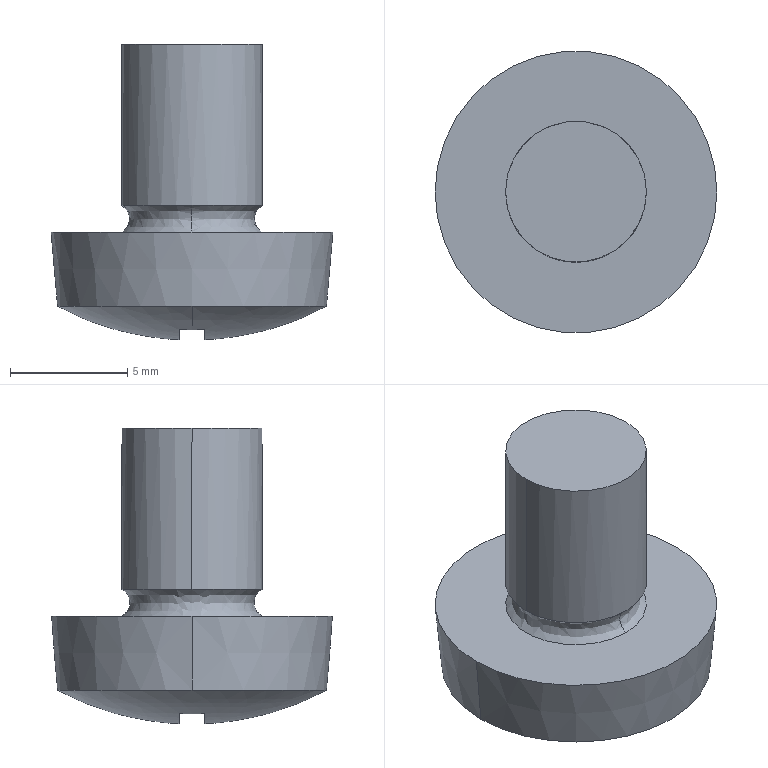Part | SolidWorks | features BaseBody 1 | 1 solid | 23 faces | box 12 x 12 x 12.575 mm | volume 614.773 mm3 | plane 15 | spline 4 | cone 2 | cylinder 2 | commonest cylinder face diameters 6 x2
STEP:
#1=CARTESIAN_POINT('',(480.537,34.715,-66.134));
#2=VERTEX_POINT('',#1);
#3=CARTESIAN_POINT('',(480.537,40.715,-66.134));
#4=VERTEX_POINT('',#3);
#5=CARTESIAN_POINT('',(480.537,37.715,-66.134));
#6=DIRECTION('',(-0.000000013,0.,1.));
#7=DIRECTION('',(-1.,0.,-0.000000013));
#8=AXIS2_PLACEMENT_3D('',#5,#6,#7);
#9=CIRCLE('',#8,3.);
#10=EDGE_CURVE('',#2,#4,#9,.T.);
#11=ORIENTED_EDGE('',*,*,#10,.T.);
#12=CARTESIAN_POINT('',(480.537,40.715,-64.991));
#13=VERTEX_POINT('',#12);
#14=CARTESIAN_POINT('',(480.537,40.715,-66.134));
#15=CARTESIAN_POINT('',(480.537,40.668,-66.111));
#16=CARTESIAN_POINT('',(480.537,40.572,-66.049));
#17=CARTESIAN_POINT('',(480.537,40.454,-65.917));
#18=CARTESIAN_POINT('',(480.537,40.375,-65.747));
#19=CARTESIAN_POINT('',(480.537,40.348,-65.563));
#20=CARTESIAN_POINT('',(480.537,40.375,-65.378));
#21=CARTESIAN_POINT('',(480.537,40.454,-65.208));
#22=CARTESIAN_POINT('',(480.537,40.572,-65.076));
#23=CARTESIAN_POINT('',(480.537,40.668,-65.014));
#24=CARTESIAN_POINT('',(480.537,40.715,-64.991));
#25=B_SPLINE_CURVE_WITH_KNOTS('',3,(#14,#15,#16,#17,#18,#19,#20,#21,#22,#23,#24),.UNSPECIFIED.,.F.,.F.,(4,1,1,1,1,1,1,1,4),(0.01923,0.125,0.25,0.375,0.5,0.625,0.75,0.875,0.9808),.UNSPECIFIED.);
#26=EDGE_CURVE('',#4,#13,#25,.T.);
#27=ORIENTED_EDGE('',*,*,#26,.T.);
#28=CARTESIAN_POINT('',(483.537,37.715,-64.991));
#29=VERTEX_POINT('',#28);
#30=CARTESIAN_POINT('',(480.537,37.715,-64.991));
#31=DIRECTION('',(0.000000013,0.,-1.));
#32=DIRECTION('',(0.,-1.,0.));
#33=AXIS2_PLACEMENT_3D('',#30,#31,#32);
#34=CIRCLE('',#33,3.);
#35=EDGE_CURVE('',#13,#29,#34,.T.);
#36=ORIENTED_EDGE('',*,*,#35,.T.);
#37=CARTESIAN_POINT('',(480.537,34.715,-64.991));
#38=VERTEX_POINT('',#37);
#39=CARTESIAN_POINT('',(480.537,37.715,-64.991));
#40=DIRECTION('',(0.000000013,0.,-1.));
#41=DIRECTION('',(0.,-1.,0.));
#42=AXIS2_PLACEMENT_3D('',#39,#40,#41);
#43=CIRCLE('',#42,3.);
#44=EDGE_CURVE('',#29,#38,#43,.T.);
#45=ORIENTED_EDGE('',*,*,#44,.T.);
#46=CARTESIAN_POINT('',(480.537,34.715,-66.134));
#47=CARTESIAN_POINT('',(480.537,34.762,-66.111));
#48=CARTESIAN_POINT('',(480.537,34.858,-66.049));
#49=CARTESIAN_POINT('',(480.537,34.976,-65.917));
#50=CARTESIAN_POINT('',(480.537,35.055,-65.747));
#51=CARTESIAN_POINT('',(480.537,35.082,-65.563));
#52=CARTESIAN_POINT('',(480.537,35.055,-65.378));
#53=CARTESIAN_POINT('',(480.537,34.976,-65.208));
#54=CARTESIAN_POINT('',(480.537,34.858,-65.076));
#55=CARTESIAN_POINT('',(480.537,34.762,-65.014));
#56=CARTESIAN_POINT('',(480.537,34.715,-64.991));
#57=B_SPLINE_CURVE_WITH_KNOTS('',3,(#46,#47,#48,#49,#50,#51,#52,#53,#54,#55,#56),.UNSPECIFIED.,.F.,.F.,(4,1,1,1,1,1,1,1,4),(0.01923,0.125,0.25,0.375,0.5,0.625,0.75,0.875,0.9808),.UNSPECIFIED.);
#58=EDGE_CURVE('',#2,#38,#57,.T.);
#59=ORIENTED_EDGE('',*,*,#58,.F.);
#60=EDGE_LOOP('',(#11,#27,#36,#45,#59));
#61=FACE_OUTER_BOUND('',#60,.T.);
#62=CARTESIAN_POINT('',(480.537,40.715,-66.134));
#63=CARTESIAN_POINT('',(482.294,40.715,-66.134));
#64=CARTESIAN_POINT('',(483.537,39.472,-66.134));
#65=CARTESIAN_POINT('',(483.537,37.715,-66.134));
#66=CARTESIAN_POINT('',(483.537,35.957,-66.134));
#67=CARTESIAN_POINT('',(482.294,34.715,-66.134));
#68=CARTESIAN_POINT('',(480.537,34.715,-66.134));
#69=CARTESIAN_POINT('',(480.537,40.668,-66.111));
#70=CARTESIAN_POINT('',(482.267,40.668,-66.111));
#71=CARTESIAN_POINT('',(483.49,39.445,-66.111));
#72=CARTESIAN_POINT('',(483.49,37.715,-66.111));
#73=CARTESIAN_POINT('',(483.49,35.985,-66.111));
#74=CARTESIAN_POINT('',(482.267,34.762,-66.111));
#75=CARTESIAN_POINT('',(480.537,34.762,-66.111));
#76=CARTESIAN_POINT('',(480.537,40.572,-66.049));
#77=CARTESIAN_POINT('',(482.21,40.572,-66.049));
#78=CARTESIAN_POINT('',(483.394,39.388,-66.049));
#79=CARTESIAN_POINT('',(483.394,37.715,-66.049));
#80=CARTESIAN_POINT('',(483.394,36.041,-66.049));
#81=CARTESIAN_POINT('',(482.21,34.858,-66.049));
#82=CARTESIAN_POINT('',(480.537,34.858,-66.049));
#83=CARTESIAN_POINT('',(480.537,40.454,-65.917));
#84=CARTESIAN_POINT('',(482.141,40.454,-65.917));
#85=CARTESIAN_POINT('',(483.276,39.319,-65.917));
#86=CARTESIAN_POINT('',(483.276,37.715,-65.917));
#87=CARTESIAN_POINT('',(483.276,36.11,-65.917));
#88=CARTESIAN_POINT('',(482.141,34.976,-65.917));
#89=CARTESIAN_POINT('',(480.537,34.976,-65.917));
#90=CARTESIAN_POINT('',(480.537,40.375,-65.747));
#91=CARTESIAN_POINT('',(482.095,40.375,-65.747));
#92=CARTESIAN_POINT('',(483.197,39.273,-65.747));
#93=CARTESIAN_POINT('',(483.197,37.715,-65.747));
#94=CARTESIAN_POINT('',(483.197,36.157,-65.747));
#95=CARTESIAN_POINT('',(482.095,35.055,-65.747));
#96=CARTESIAN_POINT('',(480.537,35.055,-65.747));
#97=CARTESIAN_POINT('',(480.537,40.348,-65.563));
#98=CARTESIAN_POINT('',(482.079,40.348,-65.563));
#99=CARTESIAN_POINT('',(483.17,39.257,-65.563));
#100=CARTESIAN_POINT('',(483.17,37.715,-65.563));
#101=CARTESIAN_POINT('',(483.17,36.172,-65.563));
#102=CARTESIAN_POINT('',(482.079,35.082,-65.563));
#103=CARTESIAN_POINT('',(480.537,35.082,-65.563));
#104=CARTESIAN_POINT('',(480.537,40.375,-65.378));
#105=CARTESIAN_POINT('',(482.095,40.375,-65.378));
#106=CARTESIAN_POINT('',(483.197,39.273,-65.378));
#107=CARTESIAN_POINT('',(483.197,37.715,-65.378));
#108=CARTESIAN_POINT('',(483.197,36.157,-65.378));
#109=CARTESIAN_POINT('',(482.095,35.055,-65.378));
#110=CARTESIAN_POINT('',(480.537,35.055,-65.378));
#111=CARTESIAN_POINT('',(480.537,40.454,-65.208));
#112=CARTESIAN_POINT('',(482.141,40.454,-65.208));
#113=CARTESIAN_POINT('',(483.276,39.319,-65.208));
#114=CARTESIAN_POINT('',(483.276,37.715,-65.208));
#115=CARTESIAN_POINT('',(483.276,36.11,-65.208));
#116=CARTESIAN_POINT('',(482.141,34.976,-65.208));
#117=CARTESIAN_POINT('',(480.537,34.976,-65.208));
#118=CARTESIAN_POINT('',(480.537,40.572,-65.076));
#119=CARTESIAN_POINT('',(482.21,40.572,-65.076));
#120=CARTESIAN_POINT('',(483.394,39.388,-65.076));
#121=CARTESIAN_POINT('',(483.394,37.715,-65.076));
#122=CARTESIAN_POINT('',(483.394,36.041,-65.076));
#123=CARTESIAN_POINT('',(482.21,34.858,-65.076));
#124=CARTESIAN_POINT('',(480.537,34.858,-65.076));
#125=CARTESIAN_POINT('',(480.537,40.668,-65.014));
#126=CARTESIAN_POINT('',(482.267,40.668,-65.014));
#127=CARTESIAN_POINT('',(483.49,39.445,-65.014));
#128=CARTESIAN_POINT('',(483.49,37.715,-65.014));
#129=CARTESIAN_POINT('',(483.49,35.985,-65.014));
#130=CARTESIAN_POINT('',(482.267,34.762,-65.014));
#131=CARTESIAN_POINT('',(480.537,34.762,-65.014));
#132=CARTESIAN_POINT('',(480.537,40.715,-64.991));
#133=CARTESIAN_POINT('',(482.294,40.715,-64.991));
#134=CARTESIAN_POINT('',(483.537,39.472,-64.991));
#135=CARTESIAN_POINT('',(483.537,37.715,-64.991));
#136=CARTESIAN_POINT('',(483.537,35.957,-64.991));
#137=CARTESIAN_POINT('',(482.294,34.715,-64.991));
#138=CARTESIAN_POINT('',(480.537,34.715,-64.991));
#139=(BOUNDED_SURFACE()B_SPLINE_SURFACE(3,3,((#62,#63,#64,#65,#66,#67,#68),(#69,#70,#71,#72,#73,#74,#75),(#76,#77,#78,#79,#80,#81,#82),(#83,#84,#85,#86,#87,#88,#89),(#90,#91,#92,#93,#94,#95,#96),(#97,#98,#99,#100,#101,#102,#103),(#104,#105,#106,#107,#108,#109,#110),(#111,#112,#113,#114,#115,#116,#117),(#118,#119,#120,#121,#122,#123,#124),(#125,#126,#127,#128,#129,#130,#131),(#132,#133,#134,#135,#136,#137,#138)),.UNSPECIFIED.,.F.,.F.,.F.)B_SPLINE_SURFACE_WITH_KNOTS((4,1,1,1,1,1,1,1,4),(4,3,4),(0.01923,0.125,0.25,0.375,0.5,0.625,0.75,0.875,0.9808),(0.,0.5,1.),.UNSPECIFIED.)GEOMETRIC_REPRESENTATION_ITEM()RATIONAL_B_SPLINE_SURFACE(((1.,0.8047,0.8047,1.,0.8047,0.8047,1.),(1.,0.8047,0.8047,1.,0.8047,0.8047,1.),(1.,0.8047,0.8047,1.,0.8047,0.8047,1.),(1.,0.8047,0.8047,1.,0.8047,0.8047,1.),(1.,0.8047,0.8047,1.,0.8047,0.8047,1.),(1.,0.8047,0.8047,1.,0.8047,0.8047,1.),(1.,0.8047,0.8047,1.,0.8047,0.8047,1.),(1.,0.8047,0.8047,1.,0.8047,0.8047,1.),(1.,0.8047,0.8047,1.,0.8047,0.8047,1.),(1.,0.8047,0.8047,1.,0.8047,0.8047,1.),(1.,0.8047,0.8047,1.,0.8047,0.8047,1.)))REPRESENTATION_ITEM('')SURFACE());
#140=ADVANCED_FACE('',(#61),#139,.T.);
#141=CARTESIAN_POINT('',(479.987,34.513,-70.286));
#142=VERTEX_POINT('',#141);
#143=CARTESIAN_POINT('',(480.537,34.503,-70.296));
#144=VERTEX_POINT('',#143);
#145=CARTESIAN_POINT('',(479.987,34.513,-70.286));
#146=CARTESIAN_POINT('',(480.17,34.506,-70.293));
#147=CARTESIAN_POINT('',(480.353,34.503,-70.296));
#148=CARTESIAN_POINT('',(480.537,34.503,-70.296));
#149=B_SPLINE_CURVE_WITH_KNOTS('',3,(#145,#146,#147,#148),.UNSPECIFIED.,.F.,.F.,(4,4),(0.,1.),.UNSPECIFIED.);
#150=EDGE_CURVE('',#142,#144,#149,.T.);
#151=ORIENTED_EDGE('',*,*,#150,.T.);
#152=CARTESIAN_POINT('',(480.537,31.99,-69.28));
#153=VERTEX_POINT('',#152);
#154=CARTESIAN_POINT('',(480.537,34.503,-70.296));
#155=CARTESIAN_POINT('',(480.537,34.464,-70.285));
#156=CARTESIAN_POINT('',(480.537,33.593,-70.039));
#157=CARTESIAN_POINT('',(480.537,32.75,-69.693));
#158=CARTESIAN_POINT('',(480.537,31.99,-69.28));
#159=B_SPLINE_CURVE_WITH_KNOTS('',3,(#154,#155,#156,#157,#158),.UNSPECIFIED.,.F.,.F.,(4,1,4),(0.4775,0.5,0.9808),.UNSPECIFIED.);
#160=EDGE_CURVE('',#144,#153,#159,.T.);
#161=ORIENTED_EDGE('',*,*,#160,.T.);
#162=CARTESIAN_POINT('',(474.812,37.715,-69.28));
#163=VERTEX_POINT('',#162);
#164=CARTESIAN_POINT('',(480.537,37.715,-69.28));
#165=DIRECTION('',(0.000000013,0.,-1.));
#166=DIRECTION('',(0.,-1.,0.));
#167=AXIS2_PLACEMENT_3D('',#164,#165,#166);
#168=CIRCLE('',#167,5.725);
#169=EDGE_CURVE('',#153,#163,#168,.T.);
#170=ORIENTED_EDGE('',*,*,#169,.T.);
#171=CARTESIAN_POINT('',(480.537,43.439,-69.28));
#172=VERTEX_POINT('',#171);
#173=CARTESIAN_POINT('',(480.537,37.715,-69.28));
#174=DIRECTION('',(0.000000013,0.,-1.));
#175=DIRECTION('',(0.,-1.,0.));
#176=AXIS2_PLACEMENT_3D('',#173,#174,#175);
#177=CIRCLE('',#176,5.725);
#178=EDGE_CURVE('',#163,#172,#177,.T.);
#179=ORIENTED_EDGE('',*,*,#178,.T.);
#180=CARTESIAN_POINT('',(480.537,40.927,-70.296));
#181=VERTEX_POINT('',#180);
#182=CARTESIAN_POINT('',(480.537,40.927,-70.296));
#183=CARTESIAN_POINT('',(480.537,40.966,-70.285));
#184=CARTESIAN_POINT('',(480.537,41.837,-70.039));
#185=CARTESIAN_POINT('',(480.537,42.679,-69.693));
#186=CARTESIAN_POINT('',(480.537,43.439,-69.28));
#187=B_SPLINE_CURVE_WITH_KNOTS('',3,(#182,#183,#184,#185,#186),.UNSPECIFIED.,.F.,.F.,(4,1,4),(0.4775,0.5,0.9808),.UNSPECIFIED.);
#188=EDGE_CURVE('',#181,#172,#187,.T.);
#189=ORIENTED_EDGE('',*,*,#188,.F.);
#190=CARTESIAN_POINT('',(479.987,40.917,-70.286));
#191=VERTEX_POINT('',#190);
#192=CARTESIAN_POINT('',(480.537,40.927,-70.296));
#193=CARTESIAN_POINT('',(480.353,40.927,-70.296));
#194=CARTESIAN_POINT('',(480.17,40.923,-70.293));
#195=CARTESIAN_POINT('',(479.987,40.917,-70.286));
#196=B_SPLINE_CURVE_WITH_KNOTS('',3,(#192,#193,#194,#195),.UNSPECIFIED.,.F.,.F.,(4,4),(0.,1.),.UNSPECIFIED.);
#197=EDGE_CURVE('',#181,#191,#196,.T.);
#198=ORIENTED_EDGE('',*,*,#197,.T.);
#199=CARTESIAN_POINT('',(479.987,38.265,-70.709));
#200=VERTEX_POINT('',#199);
#201=CARTESIAN_POINT('',(479.987,38.265,-70.709));
#202=CARTESIAN_POINT('',(479.987,39.165,-70.667));
#203=CARTESIAN_POINT('',(479.987,40.049,-70.526));
#204=CARTESIAN_POINT('',(479.987,40.917,-70.286));
#205=B_SPLINE_CURVE_WITH_KNOTS('',3,(#201,#202,#203,#204),.UNSPECIFIED.,.F.,.F.,(4,4),(0.,0.002685),.UNSPECIFIED.);
#206=EDGE_CURVE('',#200,#191,#205,.T.);
#207=ORIENTED_EDGE('',*,*,#206,.F.);
#208=CARTESIAN_POINT('',(477.335,38.265,-70.286));
#209=VERTEX_POINT('',#208);
#210=CARTESIAN_POINT('',(477.335,38.265,-70.286));
#211=CARTESIAN_POINT('',(478.203,38.265,-70.526));
#212=CARTESIAN_POINT('',(479.087,38.265,-70.667));
#213=CARTESIAN_POINT('',(479.987,38.265,-70.709));
#214=B_SPLINE_CURVE_WITH_KNOTS('',3,(#210,#211,#212,#213),.UNSPECIFIED.,.F.,.F.,(4,4),(0.,0.002685),.UNSPECIFIED.);
#215=EDGE_CURVE('',#209,#200,#214,.T.);
#216=ORIENTED_EDGE('',*,*,#215,.F.);
#217=CARTESIAN_POINT('',(477.335,37.165,-70.286));
#218=VERTEX_POINT('',#217);
#219=CARTESIAN_POINT('',(477.335,38.265,-70.286));
#220=CARTESIAN_POINT('',(477.321,37.898,-70.3));
#221=CARTESIAN_POINT('',(477.321,37.531,-70.3));
#222=CARTESIAN_POINT('',(477.335,37.165,-70.286));
#223=B_SPLINE_CURVE_WITH_KNOTS('',3,(#219,#220,#221,#222),.UNSPECIFIED.,.F.,.F.,(4,4),(0.,0.0011),.UNSPECIFIED.);
#224=EDGE_CURVE('',#209,#218,#223,.T.);
#225=ORIENTED_EDGE('',*,*,#224,.T.);
#226=CARTESIAN_POINT('',(479.987,37.165,-70.709));
#227=VERTEX_POINT('',#226);
#228=CARTESIAN_POINT('',(479.987,37.165,-70.709));
#229=CARTESIAN_POINT('',(479.087,37.165,-70.667));
#230=CARTESIAN_POINT('',(478.203,37.165,-70.526));
#231=CARTESIAN_POINT('',(477.335,37.165,-70.286));
#232=B_SPLINE_CURVE_WITH_KNOTS('',3,(#228,#229,#230,#231),.UNSPECIFIED.,.F.,.F.,(4,4),(0.,0.002685),.UNSPECIFIED.);
#233=EDGE_CURVE('',#227,#218,#232,.T.);
#234=ORIENTED_EDGE('',*,*,#233,.F.);
#235=CARTESIAN_POINT('',(479.987,34.513,-70.286));
#236=CARTESIAN_POINT('',(479.987,35.381,-70.526));
#237=CARTESIAN_POINT('',(479.987,36.265,-70.667));
#238=CARTESIAN_POINT('',(479.987,37.165,-70.709));
#239=B_SPLINE_CURVE_WITH_KNOTS('',3,(#235,#236,#237,#238),.UNSPECIFIED.,.F.,.F.,(4,4),(0.,0.002685),.UNSPECIFIED.);
#240=EDGE_CURVE('',#142,#227,#239,.T.);
#241=ORIENTED_EDGE('',*,*,#240,.F.);
#242=EDGE_LOOP('',(#151,#161,#170,#179,#189,#198,#207,#216,#225,#234,#241));
#243=FACE_OUTER_BOUND('',#242,.T.);
#244=CARTESIAN_POINT('',(480.537,38.461,-70.711));
#245=CARTESIAN_POINT('',(479.043,38.461,-70.711));
#246=CARTESIAN_POINT('',(479.043,36.968,-70.711));
#247=CARTESIAN_POINT('',(480.537,36.968,-70.711));
#248=CARTESIAN_POINT('',(480.537,39.335,-70.656));
#249=CARTESIAN_POINT('',(477.296,39.335,-70.656));
#250=CARTESIAN_POINT('',(477.296,36.094,-70.656));
#251=CARTESIAN_POINT('',(480.537,36.094,-70.656));
#252=CARTESIAN_POINT('',(480.537,41.06,-70.357));
#253=CARTESIAN_POINT('',(473.847,41.06,-70.357));
#254=CARTESIAN_POINT('',(473.847,34.37,-70.357));
#255=CARTESIAN_POINT('',(480.537,34.37,-70.357));
#256=CARTESIAN_POINT('',(480.537,42.679,-69.693));
#257=CARTESIAN_POINT('',(470.608,42.679,-69.693));
#258=CARTESIAN_POINT('',(470.608,32.75,-69.693));
#259=CARTESIAN_POINT('',(480.537,32.75,-69.693));
#260=CARTESIAN_POINT('',(480.537,43.439,-69.28));
#261=CARTESIAN_POINT('',(469.087,43.439,-69.28));
#262=CARTESIAN_POINT('',(469.087,31.99,-69.28));
#263=CARTESIAN_POINT('',(480.537,31.99,-69.28));
#264=(BOUNDED_SURFACE()B_SPLINE_SURFACE(3,3,((#244,#245,#246,#247),(#248,#249,#250,#251),(#252,#253,#254,#255),(#256,#257,#258,#259),(#260,#261,#262,#263)),.UNSPECIFIED.,.F.,.F.,.F.)B_SPLINE_SURFACE_WITH_KNOTS((4,1,4),(4,4),(0.01346,0.5,0.9808),(0.,1.),.UNSPECIFIED.)GEOMETRIC_REPRESENTATION_ITEM()RATIONAL_B_SPLINE_SURFACE(((1.,0.3333,0.3333,1.),(1.,0.3333,0.3333,1.),(1.,0.3333,0.3333,1.),(1.,0.3333,0.3333,1.),(1.,0.3333,0.3333,1.)))REPRESENTATION_ITEM('')SURFACE());
#265=ADVANCED_FACE('',(#243),#264,.F.);
#266=ORIENTED_EDGE('',*,*,#178,.F.);
#267=CARTESIAN_POINT('',(474.537,37.715,-66.134));
#268=VERTEX_POINT('',#267);
#269=CARTESIAN_POINT('',(474.537,37.715,-66.134));
#270=DIRECTION('',(-0.08716,0.,0.9962));
#271=VECTOR('',#270,1000.);
#272=LINE('',#269,#271);
#273=EDGE_CURVE('',#163,#268,#272,.T.);
#274=ORIENTED_EDGE('',*,*,#273,.T.);
#275=CARTESIAN_POINT('',(486.537,37.715,-66.134));
#276=VERTEX_POINT('',#275);
#277=CARTESIAN_POINT('',(480.537,37.715,-66.134));
#278=DIRECTION('',(0.000000013,0.,-1.));
#279=DIRECTION('',(1.,0.,0.000000013));
#280=AXIS2_PLACEMENT_3D('',#277,#278,#279);
#281=CIRCLE('',#280,6.);
#282=EDGE_CURVE('',#268,#276,#281,.T.);
#283=ORIENTED_EDGE('',*,*,#282,.T.);
#284=CARTESIAN_POINT('',(486.262,37.715,-69.28));
#285=VERTEX_POINT('',#284);
#286=CARTESIAN_POINT('',(486.537,37.715,-66.134));
#287=DIRECTION('',(0.08716,0.,0.9962));
#288=VECTOR('',#287,1000.);
#289=LINE('',#286,#288);
#290=EDGE_CURVE('',#285,#276,#289,.T.);
#291=ORIENTED_EDGE('',*,*,#290,.F.);
#292=CARTESIAN_POINT('',(480.537,37.715,-69.28));
#293=DIRECTION('',(0.000000013,0.,-1.));
#294=DIRECTION('',(0.,-1.,0.));
#295=AXIS2_PLACEMENT_3D('',#292,#293,#294);
#296=CIRCLE('',#295,5.725);
#297=EDGE_CURVE('',#172,#285,#296,.T.);
#298=ORIENTED_EDGE('',*,*,#297,.F.);
#299=EDGE_LOOP('',(#266,#274,#283,#291,#298));
#300=FACE_OUTER_BOUND('',#299,.T.);
#301=CARTESIAN_POINT('',(480.537,37.715,-66.134));
#302=DIRECTION('',(-0.000000013,0.,1.));
#303=DIRECTION('',(1.,0.,0.000000013));
#304=AXIS2_PLACEMENT_3D('',#301,#302,#303);
#305=CONICAL_SURFACE('',#304,6.,0.08727);
#306=ADVANCED_FACE('',(#300),#305,.T.);
#307=CARTESIAN_POINT('',(483.537,37.715,-58.134));
#308=VERTEX_POINT('',#307);
#309=CARTESIAN_POINT('',(477.537,37.715,-58.134));
#310=VERTEX_POINT('',#309);
#311=CARTESIAN_POINT('',(480.537,37.715,-58.134));
#312=DIRECTION('',(-0.000000013,0.,1.));
#313=DIRECTION('',(-1.,0.,-0.000000013));
#314=AXIS2_PLACEMENT_3D('',#311,#312,#313);
#315=CIRCLE('',#314,3.);
#316=EDGE_CURVE('',#308,#310,#315,.T.);
#317=ORIENTED_EDGE('',*,*,#316,.F.);
#318=CARTESIAN_POINT('',(483.537,37.715,-58.134));
#319=DIRECTION('',(0.000000013,0.,-1.));
#320=VECTOR('',#319,1000.);
#321=LINE('',#318,#320);
#322=EDGE_CURVE('',#308,#29,#321,.T.);
#323=ORIENTED_EDGE('',*,*,#322,.T.);
#324=ORIENTED_EDGE('',*,*,#35,.F.);
#325=CARTESIAN_POINT('',(477.537,37.715,-64.991));
#326=VERTEX_POINT('',#325);
#327=CARTESIAN_POINT('',(480.537,37.715,-64.991));
#328=DIRECTION('',(0.000000013,0.,-1.));
#329=DIRECTION('',(0.,-1.,0.));
#330=AXIS2_PLACEMENT_3D('',#327,#328,#329);
#331=CIRCLE('',#330,3.);
#332=EDGE_CURVE('',#326,#13,#331,.T.);
#333=ORIENTED_EDGE('',*,*,#332,.F.);
#334=CARTESIAN_POINT('',(477.537,37.715,-58.134));
#335=DIRECTION('',(0.000000013,0.,-1.));
#336=VECTOR('',#335,1000.);
#337=LINE('',#334,#336);
#338=EDGE_CURVE('',#310,#326,#337,.T.);
#339=ORIENTED_EDGE('',*,*,#338,.F.);
#340=EDGE_LOOP('',(#317,#323,#324,#333,#339));
#341=FACE_OUTER_BOUND('',#340,.T.);
#342=CARTESIAN_POINT('',(480.537,37.715,-58.134));
#343=DIRECTION('',(0.000000013,0.,-1.));
#344=DIRECTION('',(-1.,0.,-0.000000013));
#345=AXIS2_PLACEMENT_3D('',#342,#343,#344);
#346=CYLINDRICAL_SURFACE('',#345,3.);
#347=ADVANCED_FACE('',(#341),#346,.T.);
#348=ORIENTED_EDGE('',*,*,#10,.F.);
#349=CARTESIAN_POINT('',(480.537,37.715,-66.134));
#350=DIRECTION('',(-0.000000013,0.,1.));
#351=DIRECTION('',(-1.,0.,-0.000000013));
#352=AXIS2_PLACEMENT_3D('',#349,#350,#351);
#353=CIRCLE('',#352,3.);
#354=EDGE_CURVE('',#4,#2,#353,.T.);
#355=ORIENTED_EDGE('',*,*,#354,.F.);
#356=EDGE_LOOP('',(#348,#355));
#357=FACE_BOUND('',#356,.T.);
#358=CARTESIAN_POINT('',(480.537,37.715,-66.134));
#359=DIRECTION('',(0.000000013,0.,-1.));
#360=DIRECTION('',(1.,0.,0.000000013));
#361=AXIS2_PLACEMENT_3D('',#358,#359,#360);
#362=CIRCLE('',#361,6.);
#363=EDGE_CURVE('',#276,#268,#362,.T.);
#364=ORIENTED_EDGE('',*,*,#363,.F.);
#365=ORIENTED_EDGE('',*,*,#282,.F.);
#366=EDGE_LOOP('',(#364,#365));
#367=FACE_OUTER_BOUND('',#366,.T.);
#368=CARTESIAN_POINT('',(486.781,43.955,-66.134));
#369=DIRECTION('',(0.000000013,0.,-1.));
#370=DIRECTION('',(0.,-1.,0.));
#371=AXIS2_PLACEMENT_3D('',#368,#369,#370);
#372=PLANE('',#371);
#373=ADVANCED_FACE('',(#357,#367),#372,.F.);
#374=ORIENTED_EDGE('',*,*,#26,.F.);
#375=ORIENTED_EDGE('',*,*,#354,.T.);
#376=ORIENTED_EDGE('',*,*,#58,.T.);
#377=CARTESIAN_POINT('',(480.537,37.715,-64.991));
#378=DIRECTION('',(0.000000013,0.,-1.));
#379=DIRECTION('',(0.,-1.,0.));
#380=AXIS2_PLACEMENT_3D('',#377,#378,#379);
#381=CIRCLE('',#380,3.);
#382=EDGE_CURVE('',#38,#326,#381,.T.);
#383=ORIENTED_EDGE('',*,*,#382,.T.);
#384=ORIENTED_EDGE('',*,*,#332,.T.);
#385=EDGE_LOOP('',(#374,#375,#376,#383,#384));
#386=FACE_OUTER_BOUND('',#385,.T.);
#387=CARTESIAN_POINT('',(480.537,34.715,-66.134));
#388=CARTESIAN_POINT('',(478.779,34.715,-66.134));
#389=CARTESIAN_POINT('',(477.537,35.957,-66.134));
#390=CARTESIAN_POINT('',(477.537,37.715,-66.134));
#391=CARTESIAN_POINT('',(477.537,39.472,-66.134));
#392=CARTESIAN_POINT('',(478.779,40.715,-66.134));
#393=CARTESIAN_POINT('',(480.537,40.715,-66.134));
#394=CARTESIAN_POINT('',(480.537,34.762,-66.111));
#395=CARTESIAN_POINT('',(478.807,34.762,-66.111));
#396=CARTESIAN_POINT('',(477.584,35.985,-66.111));
#397=CARTESIAN_POINT('',(477.584,37.715,-66.111));
#398=CARTESIAN_POINT('',(477.584,39.445,-66.111));
#399=CARTESIAN_POINT('',(478.807,40.668,-66.111));
#400=CARTESIAN_POINT('',(480.537,40.668,-66.111));
#401=CARTESIAN_POINT('',(480.537,34.858,-66.049));
#402=CARTESIAN_POINT('',(478.863,34.858,-66.049));
#403=CARTESIAN_POINT('',(477.68,36.041,-66.049));
#404=CARTESIAN_POINT('',(477.68,37.715,-66.049));
#405=CARTESIAN_POINT('',(477.68,39.388,-66.049));
#406=CARTESIAN_POINT('',(478.863,40.572,-66.049));
#407=CARTESIAN_POINT('',(480.537,40.572,-66.049));
#408=CARTESIAN_POINT('',(480.537,34.976,-65.917));
#409=CARTESIAN_POINT('',(478.932,34.976,-65.917));
#410=CARTESIAN_POINT('',(477.798,36.11,-65.917));
#411=CARTESIAN_POINT('',(477.798,37.715,-65.917));
#412=CARTESIAN_POINT('',(477.798,39.319,-65.917));
#413=CARTESIAN_POINT('',(478.932,40.454,-65.917));
#414=CARTESIAN_POINT('',(480.537,40.454,-65.917));
#415=CARTESIAN_POINT('',(480.537,35.055,-65.747));
#416=CARTESIAN_POINT('',(478.979,35.055,-65.747));
#417=CARTESIAN_POINT('',(477.877,36.157,-65.747));
#418=CARTESIAN_POINT('',(477.877,37.715,-65.747));
#419=CARTESIAN_POINT('',(477.877,39.273,-65.747));
#420=CARTESIAN_POINT('',(478.979,40.375,-65.747));
#421=CARTESIAN_POINT('',(480.537,40.375,-65.747));
#422=CARTESIAN_POINT('',(480.537,35.082,-65.563));
#423=CARTESIAN_POINT('',(478.995,35.082,-65.563));
#424=CARTESIAN_POINT('',(477.904,36.172,-65.563));
#425=CARTESIAN_POINT('',(477.904,37.715,-65.563));
#426=CARTESIAN_POINT('',(477.904,39.257,-65.563));
#427=CARTESIAN_POINT('',(478.995,40.348,-65.563));
#428=CARTESIAN_POINT('',(480.537,40.348,-65.563));
#429=CARTESIAN_POINT('',(480.537,35.055,-65.378));
#430=CARTESIAN_POINT('',(478.979,35.055,-65.378));
#431=CARTESIAN_POINT('',(477.877,36.157,-65.378));
#432=CARTESIAN_POINT('',(477.877,37.715,-65.378));
#433=CARTESIAN_POINT('',(477.877,39.273,-65.378));
#434=CARTESIAN_POINT('',(478.979,40.375,-65.378));
#435=CARTESIAN_POINT('',(480.537,40.375,-65.378));
#436=CARTESIAN_POINT('',(480.537,34.976,-65.208));
#437=CARTESIAN_POINT('',(478.932,34.976,-65.208));
#438=CARTESIAN_POINT('',(477.798,36.11,-65.208));
#439=CARTESIAN_POINT('',(477.798,37.715,-65.208));
#440=CARTESIAN_POINT('',(477.798,39.319,-65.208));
#441=CARTESIAN_POINT('',(478.932,40.454,-65.208));
#442=CARTESIAN_POINT('',(480.537,40.454,-65.208));
#443=CARTESIAN_POINT('',(480.537,34.858,-65.076));
#444=CARTESIAN_POINT('',(478.863,34.858,-65.076));
#445=CARTESIAN_POINT('',(477.68,36.041,-65.076));
#446=CARTESIAN_POINT('',(477.68,37.715,-65.076));
#447=CARTESIAN_POINT('',(477.68,39.388,-65.076));
#448=CARTESIAN_POINT('',(478.863,40.572,-65.076));
#449=CARTESIAN_POINT('',(480.537,40.572,-65.076));
#450=CARTESIAN_POINT('',(480.537,34.762,-65.014));
#451=CARTESIAN_POINT('',(478.807,34.762,-65.014));
#452=CARTESIAN_POINT('',(477.584,35.985,-65.014));
#453=CARTESIAN_POINT('',(477.584,37.715,-65.014));
#454=CARTESIAN_POINT('',(477.584,39.445,-65.014));
#455=CARTESIAN_POINT('',(478.807,40.668,-65.014));
#456=CARTESIAN_POINT('',(480.537,40.668,-65.014));
#457=CARTESIAN_POINT('',(480.537,34.715,-64.991));
#458=CARTESIAN_POINT('',(478.78,34.715,-64.991));
#459=CARTESIAN_POINT('',(477.537,35.957,-64.991));
#460=CARTESIAN_POINT('',(477.537,37.715,-64.991));
#461=CARTESIAN_POINT('',(477.537,39.472,-64.991));
#462=CARTESIAN_POINT('',(478.78,40.715,-64.991));
#463=CARTESIAN_POINT('',(480.537,40.715,-64.991));
#464=(BOUNDED_SURFACE()B_SPLINE_SURFACE(3,3,((#387,#388,#389,#390,#391,#392,#393),(#394,#395,#396,#397,#398,#399,#400),(#401,#402,#403,#404,#405,#406,#407),(#408,#409,#410,#411,#412,#413,#414),(#415,#416,#417,#418,#419,#420,#421),(#422,#423,#424,#425,#426,#427,#428),(#429,#430,#431,#432,#433,#434,#435),(#436,#437,#438,#439,#440,#441,#442),(#443,#444,#445,#446,#447,#448,#449),(#450,#451,#452,#453,#454,#455,#456),(#457,#458,#459,#460,#461,#462,#463)),.UNSPECIFIED.,.F.,.F.,.F.)B_SPLINE_SURFACE_WITH_KNOTS((4,1,1,1,1,1,1,1,4),(4,3,4),(0.01923,0.125,0.25,0.375,0.5,0.625,0.75,0.875,0.9808),(0.,0.5,1.),.UNSPECIFIED.)GEOMETRIC_REPRESENTATION_ITEM()RATIONAL_B_SPLINE_SURFACE(((1.,0.8047,0.8047,1.,0.8047,0.8047,1.),(1.,0.8047,0.8047,1.,0.8047,0.8047,1.),(1.,0.8047,0.8047,1.,0.8047,0.8047,1.),(1.,0.8047,0.8047,1.,0.8047,0.8047,1.),(1.,0.8047,0.8047,1.,0.8047,0.8047,1.),(1.,0.8047,0.8047,1.,0.8047,0.8047,1.),(1.,0.8047,0.8047,1.,0.8047,0.8047,1.),(1.,0.8047,0.8047,1.,0.8047,0.8047,1.),(1.,0.8047,0.8047,1.,0.8047,0.8047,1.),(1.,0.8047,0.8047,1.,0.8047,0.8047,1.),(1.,0.8047,0.8047,1.,0.8047,0.8047,1.)))REPRESENTATION_ITEM('')SURFACE());
#465=ADVANCED_FACE('',(#386),#464,.T.);
#466=ORIENTED_EDGE('',*,*,#273,.F.);
#467=ORIENTED_EDGE('',*,*,#169,.F.);
#468=CARTESIAN_POINT('',(480.537,37.715,-69.28));
#469=DIRECTION('',(0.000000013,0.,-1.));
#470=DIRECTION('',(0.,-1.,0.));
#471=AXIS2_PLACEMENT_3D('',#468,#469,#470);
#472=CIRCLE('',#471,5.725);
#473=EDGE_CURVE('',#285,#153,#472,.T.);
#474=ORIENTED_EDGE('',*,*,#473,.F.);
#475=ORIENTED_EDGE('',*,*,#290,.T.);
#476=ORIENTED_EDGE('',*,*,#363,.T.);
#477=EDGE_LOOP('',(#466,#467,#474,#475,#476));
#478=FACE_OUTER_BOUND('',#477,.T.);
#479=CARTESIAN_POINT('',(480.537,37.715,-66.134));
#480=DIRECTION('',(-0.000000013,0.,1.));
#481=DIRECTION('',(1.,0.,0.000000013));
#482=AXIS2_PLACEMENT_3D('',#479,#480,#481);
#483=CONICAL_SURFACE('',#482,6.,0.08727);
#484=ADVANCED_FACE('',(#478),#483,.T.);
#485=ORIENTED_EDGE('',*,*,#322,.F.);
#486=CARTESIAN_POINT('',(480.537,37.715,-58.134));
#487=DIRECTION('',(-0.000000013,0.,1.));
#488=DIRECTION('',(-1.,0.,-0.000000013));
#489=AXIS2_PLACEMENT_3D('',#486,#487,#488);
#490=CIRCLE('',#489,3.);
#491=EDGE_CURVE('',#310,#308,#490,.T.);
#492=ORIENTED_EDGE('',*,*,#491,.F.);
#493=ORIENTED_EDGE('',*,*,#338,.T.);
#494=ORIENTED_EDGE('',*,*,#382,.F.);
#495=ORIENTED_EDGE('',*,*,#44,.F.);
#496=EDGE_LOOP('',(#485,#492,#493,#494,#495));
#497=FACE_OUTER_BOUND('',#496,.T.);
#498=CARTESIAN_POINT('',(480.537,37.715,-58.134));
#499=DIRECTION('',(0.000000013,0.,-1.));
#500=DIRECTION('',(-1.,0.,-0.000000013));
#501=AXIS2_PLACEMENT_3D('',#498,#499,#500);
#502=CYLINDRICAL_SURFACE('',#501,3.);
#503=ADVANCED_FACE('',(#497),#502,.T.);
#504=ORIENTED_EDGE('',*,*,#160,.F.);
#505=CARTESIAN_POINT('',(481.087,34.513,-70.286));
#506=VERTEX_POINT('',#505);
#507=CARTESIAN_POINT('',(480.537,34.503,-70.296));
#508=CARTESIAN_POINT('',(480.72,34.503,-70.296));
#509=CARTESIAN_POINT('',(480.904,34.506,-70.293));
#510=CARTESIAN_POINT('',(481.087,34.513,-70.286));
#511=B_SPLINE_CURVE_WITH_KNOTS('',3,(#507,#508,#509,#510),.UNSPECIFIED.,.F.,.F.,(4,4),(0.,1.),.UNSPECIFIED.);
#512=EDGE_CURVE('',#144,#506,#511,.T.);
#513=ORIENTED_EDGE('',*,*,#512,.T.);
#514=CARTESIAN_POINT('',(481.087,37.165,-70.709));
#515=VERTEX_POINT('',#514);
#516=CARTESIAN_POINT('',(481.087,37.165,-70.709));
#517=CARTESIAN_POINT('',(481.087,36.265,-70.667));
#518=CARTESIAN_POINT('',(481.087,35.381,-70.526));
#519=CARTESIAN_POINT('',(481.087,34.513,-70.286));
#520=B_SPLINE_CURVE_WITH_KNOTS('',3,(#516,#517,#518,#519),.UNSPECIFIED.,.F.,.F.,(4,4),(0.,0.002685),.UNSPECIFIED.);
#521=EDGE_CURVE('',#515,#506,#520,.T.);
#522=ORIENTED_EDGE('',*,*,#521,.F.);
#523=CARTESIAN_POINT('',(483.739,37.165,-70.286));
#524=VERTEX_POINT('',#523);
#525=CARTESIAN_POINT('',(483.739,37.165,-70.286));
#526=CARTESIAN_POINT('',(482.871,37.165,-70.526));
#527=CARTESIAN_POINT('',(481.987,37.165,-70.667));
#528=CARTESIAN_POINT('',(481.087,37.165,-70.709));
#529=B_SPLINE_CURVE_WITH_KNOTS('',3,(#525,#526,#527,#528),.UNSPECIFIED.,.F.,.F.,(4,4),(0.,0.002685),.UNSPECIFIED.);
#530=EDGE_CURVE('',#524,#515,#529,.T.);
#531=ORIENTED_EDGE('',*,*,#530,.F.);
#532=CARTESIAN_POINT('',(483.739,38.265,-70.286));
#533=VERTEX_POINT('',#532);
#534=CARTESIAN_POINT('',(483.739,37.165,-70.286));
#535=CARTESIAN_POINT('',(483.752,37.531,-70.3));
#536=CARTESIAN_POINT('',(483.752,37.898,-70.3));
#537=CARTESIAN_POINT('',(483.739,38.265,-70.286));
#538=B_SPLINE_CURVE_WITH_KNOTS('',3,(#534,#535,#536,#537),.UNSPECIFIED.,.F.,.F.,(4,4),(0.,0.0011),.UNSPECIFIED.);
#539=EDGE_CURVE('',#524,#533,#538,.T.);
#540=ORIENTED_EDGE('',*,*,#539,.T.);
#541=CARTESIAN_POINT('',(481.087,38.265,-70.709));
#542=VERTEX_POINT('',#541);
#543=CARTESIAN_POINT('',(481.087,38.265,-70.709));
#544=CARTESIAN_POINT('',(481.987,38.265,-70.667));
#545=CARTESIAN_POINT('',(482.871,38.265,-70.526));
#546=CARTESIAN_POINT('',(483.739,38.265,-70.286));
#547=B_SPLINE_CURVE_WITH_KNOTS('',3,(#543,#544,#545,#546),.UNSPECIFIED.,.F.,.F.,(4,4),(0.,0.002685),.UNSPECIFIED.);
#548=EDGE_CURVE('',#542,#533,#547,.T.);
#549=ORIENTED_EDGE('',*,*,#548,.F.);
#550=CARTESIAN_POINT('',(481.087,40.917,-70.286));
#551=VERTEX_POINT('',#550);
#552=CARTESIAN_POINT('',(481.087,40.917,-70.286));
#553=CARTESIAN_POINT('',(481.087,40.049,-70.526));
#554=CARTESIAN_POINT('',(481.087,39.165,-70.667));
#555=CARTESIAN_POINT('',(481.087,38.265,-70.709));
#556=B_SPLINE_CURVE_WITH_KNOTS('',3,(#552,#553,#554,#555),.UNSPECIFIED.,.F.,.F.,(4,4),(0.,0.002685),.UNSPECIFIED.);
#557=EDGE_CURVE('',#551,#542,#556,.T.);
#558=ORIENTED_EDGE('',*,*,#557,.F.);
#559=CARTESIAN_POINT('',(481.087,40.917,-70.286));
#560=CARTESIAN_POINT('',(480.904,40.923,-70.293));
#561=CARTESIAN_POINT('',(480.72,40.927,-70.296));
#562=CARTESIAN_POINT('',(480.537,40.927,-70.296));
#563=B_SPLINE_CURVE_WITH_KNOTS('',3,(#559,#560,#561,#562),.UNSPECIFIED.,.F.,.F.,(4,4),(0.,1.),.UNSPECIFIED.);
#564=EDGE_CURVE('',#551,#181,#563,.T.);
#565=ORIENTED_EDGE('',*,*,#564,.T.);
#566=ORIENTED_EDGE('',*,*,#188,.T.);
#567=ORIENTED_EDGE('',*,*,#297,.T.);
#568=ORIENTED_EDGE('',*,*,#473,.T.);
#569=EDGE_LOOP('',(#504,#513,#522,#531,#540,#549,#558,#565,#566,#567,#568));
#570=FACE_OUTER_BOUND('',#569,.T.);
#571=CARTESIAN_POINT('',(480.537,36.968,-70.711));
#572=CARTESIAN_POINT('',(482.03,36.968,-70.711));
#573=CARTESIAN_POINT('',(482.03,38.461,-70.711));
#574=CARTESIAN_POINT('',(480.537,38.461,-70.711));
#575=CARTESIAN_POINT('',(480.537,36.094,-70.656));
#576=CARTESIAN_POINT('',(483.777,36.094,-70.656));
#577=CARTESIAN_POINT('',(483.777,39.335,-70.656));
#578=CARTESIAN_POINT('',(480.537,39.335,-70.656));
#579=CARTESIAN_POINT('',(480.537,34.37,-70.357));
#580=CARTESIAN_POINT('',(487.227,34.37,-70.357));
#581=CARTESIAN_POINT('',(487.227,41.06,-70.357));
#582=CARTESIAN_POINT('',(480.537,41.06,-70.357));
#583=CARTESIAN_POINT('',(480.537,32.75,-69.693));
#584=CARTESIAN_POINT('',(490.466,32.75,-69.693));
#585=CARTESIAN_POINT('',(490.466,42.679,-69.693));
#586=CARTESIAN_POINT('',(480.537,42.679,-69.693));
#587=CARTESIAN_POINT('',(480.537,31.99,-69.28));
#588=CARTESIAN_POINT('',(491.986,31.99,-69.28));
#589=CARTESIAN_POINT('',(491.986,43.439,-69.28));
#590=CARTESIAN_POINT('',(480.537,43.439,-69.28));
#591=(BOUNDED_SURFACE()B_SPLINE_SURFACE(3,3,((#571,#572,#573,#574),(#575,#576,#577,#578),(#579,#580,#581,#582),(#583,#584,#585,#586),(#587,#588,#589,#590)),.UNSPECIFIED.,.F.,.F.,.F.)B_SPLINE_SURFACE_WITH_KNOTS((4,1,4),(4,4),(0.01346,0.5,0.9808),(0.,1.),.UNSPECIFIED.)GEOMETRIC_REPRESENTATION_ITEM()RATIONAL_B_SPLINE_SURFACE(((1.,0.3333,0.3333,1.),(1.,0.3333,0.3333,1.),(1.,0.3333,0.3333,1.),(1.,0.3333,0.3333,1.),(1.,0.3333,0.3333,1.)))REPRESENTATION_ITEM('')SURFACE());
#592=ADVANCED_FACE('',(#570),#591,.F.);
#593=ORIENTED_EDGE('',*,*,#491,.T.);
#594=ORIENTED_EDGE('',*,*,#316,.T.);
#595=EDGE_LOOP('',(#593,#594));
#596=FACE_OUTER_BOUND('',#595,.T.);
#597=CARTESIAN_POINT('',(483.66,40.835,-58.134));
#598=DIRECTION('',(0.000000013,0.,-1.));
#599=DIRECTION('',(0.,-1.,0.));
#600=AXIS2_PLACEMENT_3D('',#597,#598,#599);
#601=PLANE('',#600);
#602=ADVANCED_FACE('',(#596),#601,.F.);
#603=CARTESIAN_POINT('',(479.987,38.265,-67.634));
#604=VERTEX_POINT('',#603);
#605=CARTESIAN_POINT('',(479.987,40.917,-70.286));
#606=DIRECTION('',(-0.000000009,-0.7071,0.7071));
#607=VECTOR('',#606,1000.);
#608=LINE('',#605,#607);
#609=EDGE_CURVE('',#191,#604,#608,.T.);
#610=ORIENTED_EDGE('',*,*,#609,.T.);
#611=CARTESIAN_POINT('',(479.987,38.265,-69.171));
#612=DIRECTION('',(0.000000013,0.,-1.));
#613=VECTOR('',#612,1000.);
#614=LINE('',#611,#613);
#615=EDGE_CURVE('',#604,#200,#614,.T.);
#616=ORIENTED_EDGE('',*,*,#615,.T.);
#617=ORIENTED_EDGE('',*,*,#206,.T.);
#618=EDGE_LOOP('',(#610,#616,#617));
#619=FACE_OUTER_BOUND('',#618,.T.);
#620=CARTESIAN_POINT('',(479.987,34.385,-67.573));
#621=DIRECTION('',(1.,0.,0.000000013));
#622=DIRECTION('',(0.000000013,0.,-1.));
#623=AXIS2_PLACEMENT_3D('',#620,#621,#622);
#624=PLANE('',#623);
#625=ADVANCED_FACE('',(#619),#624,.T.);
#626=ORIENTED_EDGE('',*,*,#615,.F.);
#627=CARTESIAN_POINT('',(479.987,38.265,-67.634));
#628=DIRECTION('',(-0.7071,0.,-0.7071));
#629=VECTOR('',#628,1000.);
#630=LINE('',#627,#629);
#631=EDGE_CURVE('',#604,#209,#630,.T.);
#632=ORIENTED_EDGE('',*,*,#631,.T.);
#633=ORIENTED_EDGE('',*,*,#215,.T.);
#634=EDGE_LOOP('',(#626,#632,#633));
#635=FACE_OUTER_BOUND('',#634,.T.);
#636=CARTESIAN_POINT('',(477.207,38.265,-67.573));
#637=DIRECTION('',(0.,-1.,0.));
#638=DIRECTION('',(0.000000013,0.,-1.));
#639=AXIS2_PLACEMENT_3D('',#636,#637,#638);
#640=PLANE('',#639);
#641=ADVANCED_FACE('',(#635),#640,.T.);
#642=CARTESIAN_POINT('',(479.987,37.165,-67.634));
#643=VERTEX_POINT('',#642);
#644=CARTESIAN_POINT('',(480.04,37.165,-67.581));
#645=DIRECTION('',(-0.7071,0.,-0.7071));
#646=VECTOR('',#645,1000.);
#647=LINE('',#644,#646);
#648=EDGE_CURVE('',#643,#218,#647,.T.);
#649=ORIENTED_EDGE('',*,*,#648,.F.);
#650=CARTESIAN_POINT('',(479.987,37.165,-69.171));
#651=DIRECTION('',(-0.000000013,0.,1.));
#652=VECTOR('',#651,1000.);
#653=LINE('',#650,#652);
#654=EDGE_CURVE('',#227,#643,#653,.T.);
#655=ORIENTED_EDGE('',*,*,#654,.F.);
#656=ORIENTED_EDGE('',*,*,#233,.T.);
#657=EDGE_LOOP('',(#649,#655,#656));
#658=FACE_OUTER_BOUND('',#657,.T.);
#659=CARTESIAN_POINT('',(477.207,37.165,-67.573));
#660=DIRECTION('',(0.,-1.,0.));
#661=DIRECTION('',(0.000000013,0.,-1.));
#662=AXIS2_PLACEMENT_3D('',#659,#660,#661);
#663=PLANE('',#662);
#664=ADVANCED_FACE('',(#658),#663,.F.);
#665=ORIENTED_EDGE('',*,*,#654,.T.);
#666=CARTESIAN_POINT('',(479.987,37.165,-67.634));
#667=DIRECTION('',(0.000000009,-0.7071,-0.7071));
#668=VECTOR('',#667,1000.);
#669=LINE('',#666,#668);
#670=EDGE_CURVE('',#643,#142,#669,.T.);
#671=ORIENTED_EDGE('',*,*,#670,.T.);
#672=ORIENTED_EDGE('',*,*,#240,.T.);
#673=EDGE_LOOP('',(#665,#671,#672));
#674=FACE_OUTER_BOUND('',#673,.T.);
#675=CARTESIAN_POINT('',(479.987,34.385,-67.573));
#676=DIRECTION('',(1.,0.,0.000000013));
#677=DIRECTION('',(0.000000013,0.,-1.));
#678=AXIS2_PLACEMENT_3D('',#675,#676,#677);
#679=PLANE('',#678);
#680=ADVANCED_FACE('',(#674),#679,.T.);
#681=CARTESIAN_POINT('',(481.087,37.165,-67.634));
#682=VERTEX_POINT('',#681);
#683=CARTESIAN_POINT('',(481.087,37.218,-67.581));
#684=DIRECTION('',(0.000000009,-0.7071,-0.7071));
#685=VECTOR('',#684,1000.);
#686=LINE('',#683,#685);
#687=EDGE_CURVE('',#682,#506,#686,.T.);
#688=ORIENTED_EDGE('',*,*,#687,.F.);
#689=CARTESIAN_POINT('',(481.087,37.165,-69.171));
#690=DIRECTION('',(-0.000000013,0.,1.));
#691=VECTOR('',#690,1000.);
#692=LINE('',#689,#691);
#693=EDGE_CURVE('',#515,#682,#692,.T.);
#694=ORIENTED_EDGE('',*,*,#693,.F.);
#695=ORIENTED_EDGE('',*,*,#521,.T.);
#696=EDGE_LOOP('',(#688,#694,#695));
#697=FACE_OUTER_BOUND('',#696,.T.);
#698=CARTESIAN_POINT('',(481.087,34.385,-67.573));
#699=DIRECTION('',(1.,0.,0.000000013));
#700=DIRECTION('',(0.000000013,0.,-1.));
#701=AXIS2_PLACEMENT_3D('',#698,#699,#700);
#702=PLANE('',#701);
#703=ADVANCED_FACE('',(#697),#702,.F.);
#704=ORIENTED_EDGE('',*,*,#693,.T.);
#705=CARTESIAN_POINT('',(483.802,37.165,-70.349));
#706=DIRECTION('',(-0.7071,0.,0.7071));
#707=VECTOR('',#706,1000.);
#708=LINE('',#705,#707);
#709=EDGE_CURVE('',#524,#682,#708,.T.);
#710=ORIENTED_EDGE('',*,*,#709,.F.);
#711=ORIENTED_EDGE('',*,*,#530,.T.);
#712=EDGE_LOOP('',(#704,#710,#711));
#713=FACE_OUTER_BOUND('',#712,.T.);
#714=CARTESIAN_POINT('',(477.207,37.165,-67.573));
#715=DIRECTION('',(0.,-1.,0.));
#716=DIRECTION('',(0.000000013,0.,-1.));
#717=AXIS2_PLACEMENT_3D('',#714,#715,#716);
#718=PLANE('',#717);
#719=ADVANCED_FACE('',(#713),#718,.F.);
#720=CARTESIAN_POINT('',(481.087,38.265,-67.634));
#721=VERTEX_POINT('',#720);
#722=CARTESIAN_POINT('',(483.739,38.265,-70.286));
#723=DIRECTION('',(-0.7071,0.,0.7071));
#724=VECTOR('',#723,1000.);
#725=LINE('',#722,#724);
#726=EDGE_CURVE('',#533,#721,#725,.T.);
#727=ORIENTED_EDGE('',*,*,#726,.T.);
#728=CARTESIAN_POINT('',(481.087,38.265,-69.171));
#729=DIRECTION('',(0.000000013,0.,-1.));
#730=VECTOR('',#729,1000.);
#731=LINE('',#728,#730);
#732=EDGE_CURVE('',#721,#542,#731,.T.);
#733=ORIENTED_EDGE('',*,*,#732,.T.);
#734=ORIENTED_EDGE('',*,*,#548,.T.);
#735=EDGE_LOOP('',(#727,#733,#734));
#736=FACE_OUTER_BOUND('',#735,.T.);
#737=CARTESIAN_POINT('',(477.207,38.265,-67.573));
#738=DIRECTION('',(0.,-1.,0.));
#739=DIRECTION('',(0.000000013,0.,-1.));
#740=AXIS2_PLACEMENT_3D('',#737,#738,#739);
#741=PLANE('',#740);
#742=ADVANCED_FACE('',(#736),#741,.T.);
#743=ORIENTED_EDGE('',*,*,#732,.F.);
#744=CARTESIAN_POINT('',(481.087,40.98,-70.349));
#745=DIRECTION('',(-0.000000009,-0.7071,0.7071));
#746=VECTOR('',#745,1000.);
#747=LINE('',#744,#746);
#748=EDGE_CURVE('',#551,#721,#747,.T.);
#749=ORIENTED_EDGE('',*,*,#748,.F.);
#750=ORIENTED_EDGE('',*,*,#557,.T.);
#751=EDGE_LOOP('',(#743,#749,#750));
#752=FACE_OUTER_BOUND('',#751,.T.);
#753=CARTESIAN_POINT('',(481.087,34.385,-67.573));
#754=DIRECTION('',(1.,0.,0.000000013));
#755=DIRECTION('',(0.000000013,0.,-1.));
#756=AXIS2_PLACEMENT_3D('',#753,#754,#755);
#757=PLANE('',#756);
#758=ADVANCED_FACE('',(#752),#757,.F.);
#759=ORIENTED_EDGE('',*,*,#564,.F.);
#760=ORIENTED_EDGE('',*,*,#748,.T.);
#761=CARTESIAN_POINT('',(480.537,38.265,-67.634));
#762=DIRECTION('',(1.,0.,0.000000013));
#763=VECTOR('',#762,1000.);
#764=LINE('',#761,#763);
#765=EDGE_CURVE('',#604,#721,#764,.T.);
#766=ORIENTED_EDGE('',*,*,#765,.F.);
#767=ORIENTED_EDGE('',*,*,#609,.F.);
#768=ORIENTED_EDGE('',*,*,#197,.F.);
#769=EDGE_LOOP('',(#759,#760,#766,#767,#768));
#770=FACE_OUTER_BOUND('',#769,.T.);
#771=CARTESIAN_POINT('',(479.961,40.98,-70.349));
#772=DIRECTION('',(-0.000000009,0.7071,0.7071));
#773=DIRECTION('',(-0.000000009,-0.7071,0.7071));
#774=AXIS2_PLACEMENT_3D('',#771,#772,#773);
#775=PLANE('',#774);
#776=ADVANCED_FACE('',(#770),#775,.F.);
#777=ORIENTED_EDGE('',*,*,#631,.F.);
#778=CARTESIAN_POINT('',(479.987,37.715,-67.634));
#779=DIRECTION('',(0.,1.,0.));
#780=VECTOR('',#779,1000.);
#781=LINE('',#778,#780);
#782=EDGE_CURVE('',#643,#604,#781,.T.);
#783=ORIENTED_EDGE('',*,*,#782,.F.);
#784=ORIENTED_EDGE('',*,*,#648,.T.);
#785=ORIENTED_EDGE('',*,*,#224,.F.);
#786=EDGE_LOOP('',(#777,#783,#784,#785));
#787=FACE_OUTER_BOUND('',#786,.T.);
#788=CARTESIAN_POINT('',(480.04,38.29,-67.581));
#789=DIRECTION('',(-0.7071,0.,0.7071));
#790=DIRECTION('',(-0.7071,0.,-0.7071));
#791=AXIS2_PLACEMENT_3D('',#788,#789,#790);
#792=PLANE('',#791);
#793=ADVANCED_FACE('',(#787),#792,.F.);
#794=ORIENTED_EDGE('',*,*,#670,.F.);
#795=CARTESIAN_POINT('',(480.537,37.165,-67.634));
#796=DIRECTION('',(-1.,0.,-0.000000013));
#797=VECTOR('',#796,1000.);
#798=LINE('',#795,#797);
#799=EDGE_CURVE('',#682,#643,#798,.T.);
#800=ORIENTED_EDGE('',*,*,#799,.F.);
#801=ORIENTED_EDGE('',*,*,#687,.T.);
#802=ORIENTED_EDGE('',*,*,#512,.F.);
#803=ORIENTED_EDGE('',*,*,#150,.F.);
#804=EDGE_LOOP('',(#794,#800,#801,#802,#803));
#805=FACE_OUTER_BOUND('',#804,.T.);
#806=CARTESIAN_POINT('',(479.961,37.218,-67.581));
#807=DIRECTION('',(-0.000000009,-0.7071,0.7071));
#808=DIRECTION('',(0.000000009,-0.7071,-0.7071));
#809=AXIS2_PLACEMENT_3D('',#806,#807,#808);
#810=PLANE('',#809);
#811=ADVANCED_FACE('',(#805),#810,.F.);
#812=ORIENTED_EDGE('',*,*,#709,.T.);
#813=CARTESIAN_POINT('',(481.087,37.715,-67.634));
#814=DIRECTION('',(0.,-1.,0.));
#815=VECTOR('',#814,1000.);
#816=LINE('',#813,#815);
#817=EDGE_CURVE('',#721,#682,#816,.T.);
#818=ORIENTED_EDGE('',*,*,#817,.F.);
#819=ORIENTED_EDGE('',*,*,#726,.F.);
#820=ORIENTED_EDGE('',*,*,#539,.F.);
#821=EDGE_LOOP('',(#812,#818,#819,#820));
#822=FACE_OUTER_BOUND('',#821,.T.);
#823=CARTESIAN_POINT('',(483.802,38.29,-70.349));
#824=DIRECTION('',(0.7071,0.,0.7071));
#825=DIRECTION('',(-0.7071,0.,0.7071));
#826=AXIS2_PLACEMENT_3D('',#823,#824,#825);
#827=PLANE('',#826);
#828=ADVANCED_FACE('',(#822),#827,.F.);
#829=ORIENTED_EDGE('',*,*,#765,.T.);
#830=ORIENTED_EDGE('',*,*,#817,.T.);
#831=ORIENTED_EDGE('',*,*,#799,.T.);
#832=ORIENTED_EDGE('',*,*,#782,.T.);
#833=EDGE_LOOP('',(#829,#830,#831,#832));
#834=FACE_OUTER_BOUND('',#833,.T.);
#835=CARTESIAN_POINT('',(479.961,38.29,-67.634));
#836=DIRECTION('',(-0.000000013,0.,1.));
#837=DIRECTION('',(0.,-1.,0.));
#838=AXIS2_PLACEMENT_3D('',#835,#836,#837);
#839=PLANE('',#838);
#840=ADVANCED_FACE('',(#834),#839,.F.);
#841=CLOSED_SHELL('',(#140,#265,#306,#347,#373,#465,#484,#503,#592,#602,#625,#641,#664,#680,#703,#719,#742,#758,#776,#793,#811,#828,#840));
#842=MANIFOLD_SOLID_BREP('',#841);
#843=CARTESIAN_POINT('',(0.,0.,0.));
#844=DIRECTION('',(0.,0.,1.));
#845=DIRECTION('',(1.,0.,0.));
#846=AXIS2_PLACEMENT_3D('',#843,#844,#845);
#847=(LENGTH_UNIT()NAMED_UNIT(*)SI_UNIT(.MILLI.,.METRE.));
#848=UNCERTAINTY_MEASURE_WITH_UNIT(LENGTH_MEASURE(0.00001),#847,'','');
#849=(NAMED_UNIT(*)PLANE_ANGLE_UNIT()SI_UNIT($,.RADIAN.));
#850=(NAMED_UNIT(*)SI_UNIT($,.STERADIAN.)SOLID_ANGLE_UNIT());
#851=(GEOMETRIC_REPRESENTATION_CONTEXT(3)GLOBAL_UNCERTAINTY_ASSIGNED_CONTEXT((#848))GLOBAL_UNIT_ASSIGNED_CONTEXT((#847,#849,#850))REPRESENTATION_CONTEXT('',''));
#852=ADVANCED_BREP_SHAPE_REPRESENTATION('',(#842,#846),#851);